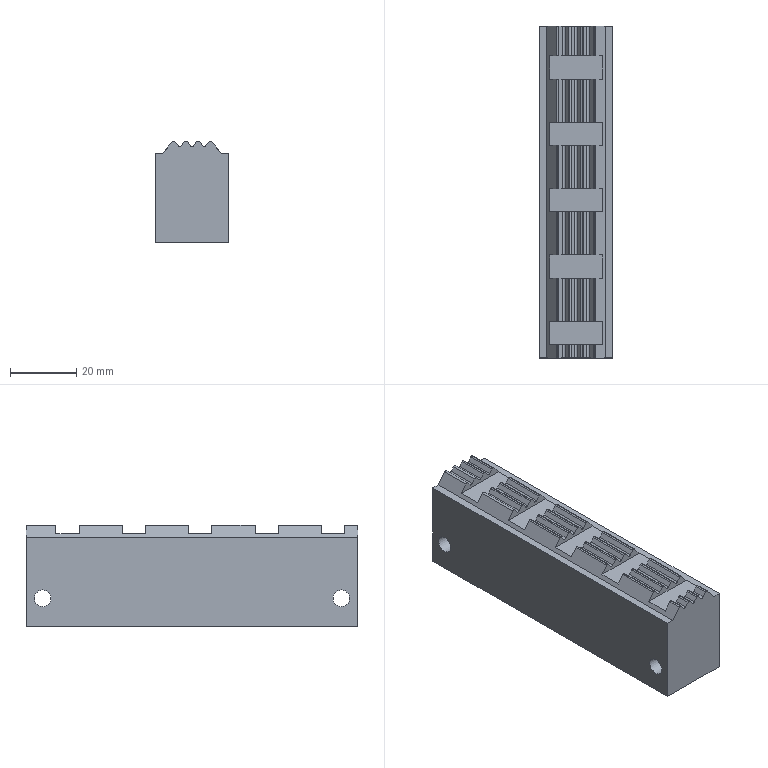Part | STEP file | 200 mesh_id1918 | 1 solid | 146 faces | box 22 x 100 x 30.627 mm | volume 61945 mm3 | plane 81 | cylinder 65 | commonest cylinder face diameters 1.04 x45 1.2 x18 5.02 x2